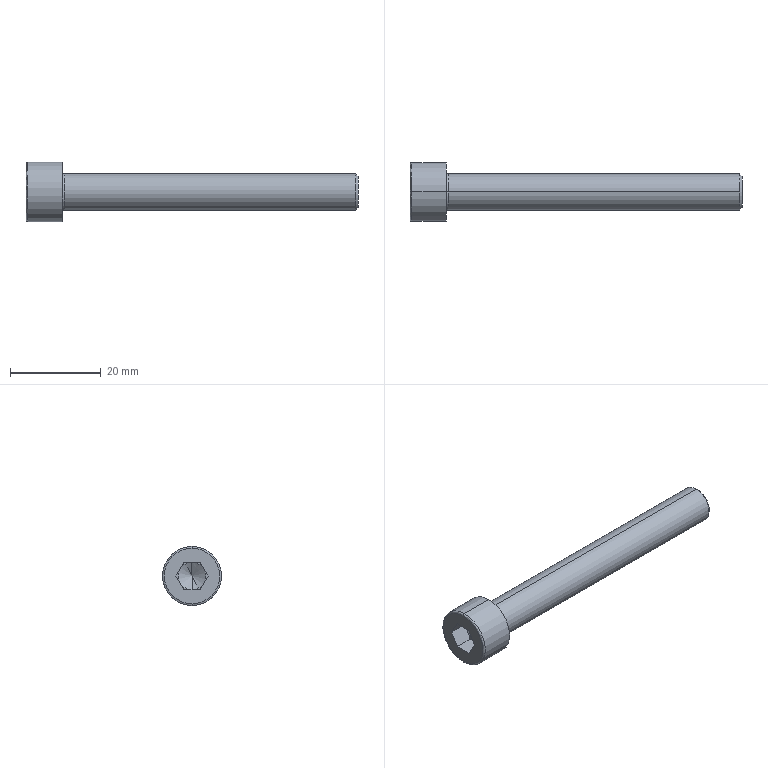Part | STEP file | PN_0029_default | 1 solid | 27 faces | box 73 x 13 x 13 mm | volume 4180 mm3 | plane 15 | spline 4 | cone 4 | cylinder 4 | commonest cylinder face diameters 8 x2 13 x2